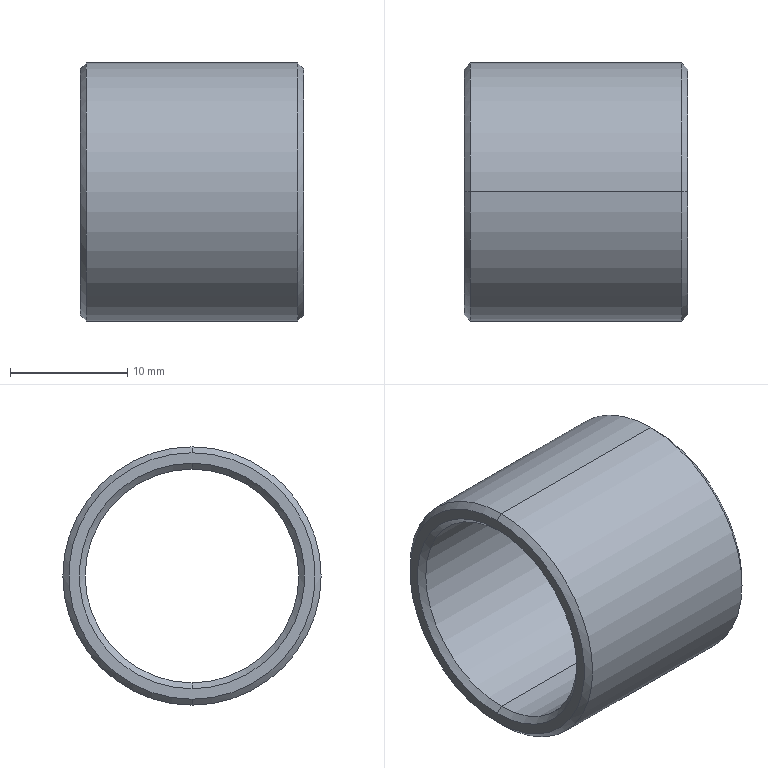Part | SolidWorks | features BaseBody 1 | 1 solid | 14 faces | box 19 x 22 x 22 mm | volume 2248 mm3 | cone 8 | cylinder 4 | plane 2 | commonest cylinder face diameters 18.2 x2 22 x2
STEP:
#1=CARTESIAN_POINT('',(100.647,1932.,-359.));
#2=VERTEX_POINT('',#1);
#3=CARTESIAN_POINT('',(100.647,1932.,-337.));
#4=VERTEX_POINT('',#3);
#5=CARTESIAN_POINT('',(100.647,1932.,-348.));
#6=DIRECTION('',(1.,0.,0.));
#7=DIRECTION('',(0.,0.,-1.));
#8=AXIS2_PLACEMENT_3D('',#5,#6,#7);
#9=CIRCLE('',#8,11.);
#10=EDGE_CURVE('',#2,#4,#9,.T.);
#11=ORIENTED_EDGE('',*,*,#10,.T.);
#12=CARTESIAN_POINT('',(118.647,1932.,-337.));
#13=VERTEX_POINT('',#12);
#14=CARTESIAN_POINT('',(100.147,1932.,-337.));
#15=DIRECTION('',(1.,0.,0.));
#16=VECTOR('',#15,1000.);
#17=LINE('',#14,#16);
#18=EDGE_CURVE('',#4,#13,#17,.T.);
#19=ORIENTED_EDGE('',*,*,#18,.T.);
#20=CARTESIAN_POINT('',(118.647,1932.,-359.));
#21=VERTEX_POINT('',#20);
#22=CARTESIAN_POINT('',(118.647,1932.,-348.));
#23=DIRECTION('',(-1.,0.,0.));
#24=DIRECTION('',(0.,0.,-1.));
#25=AXIS2_PLACEMENT_3D('',#22,#23,#24);
#26=CIRCLE('',#25,11.);
#27=EDGE_CURVE('',#13,#21,#26,.T.);
#28=ORIENTED_EDGE('',*,*,#27,.T.);
#29=CARTESIAN_POINT('',(100.147,1932.,-359.));
#30=DIRECTION('',(1.,0.,0.));
#31=VECTOR('',#30,1000.);
#32=LINE('',#29,#31);
#33=EDGE_CURVE('',#2,#21,#32,.T.);
#34=ORIENTED_EDGE('',*,*,#33,.F.);
#35=EDGE_LOOP('',(#11,#19,#28,#34));
#36=FACE_OUTER_BOUND('',#35,.T.);
#37=CARTESIAN_POINT('',(100.147,1932.,-348.));
#38=DIRECTION('',(1.,0.,0.));
#39=DIRECTION('',(0.,0.,-1.));
#40=AXIS2_PLACEMENT_3D('',#37,#38,#39);
#41=CYLINDRICAL_SURFACE('',#40,11.);
#42=ADVANCED_FACE('',(#36),#41,.T.);
#43=CARTESIAN_POINT('',(119.147,1932.,-337.5));
#44=VERTEX_POINT('',#43);
#45=CARTESIAN_POINT('',(119.147,1932.,-358.5));
#46=VERTEX_POINT('',#45);
#47=CARTESIAN_POINT('',(119.147,1932.,-348.));
#48=DIRECTION('',(-1.,0.,0.));
#49=DIRECTION('',(0.,0.,1.));
#50=AXIS2_PLACEMENT_3D('',#47,#48,#49);
#51=CIRCLE('',#50,10.5);
#52=EDGE_CURVE('',#44,#46,#51,.T.);
#53=ORIENTED_EDGE('',*,*,#52,.T.);
#54=CARTESIAN_POINT('',(118.647,1932.,-359.));
#55=DIRECTION('',(-0.7071,0.,-0.7071));
#56=VECTOR('',#55,1000.);
#57=LINE('',#54,#56);
#58=EDGE_CURVE('',#46,#21,#57,.T.);
#59=ORIENTED_EDGE('',*,*,#58,.T.);
#60=ORIENTED_EDGE('',*,*,#27,.F.);
#61=CARTESIAN_POINT('',(118.647,1932.,-337.));
#62=DIRECTION('',(-0.7071,0.,0.7071));
#63=VECTOR('',#62,1000.);
#64=LINE('',#61,#63);
#65=EDGE_CURVE('',#44,#13,#64,.T.);
#66=ORIENTED_EDGE('',*,*,#65,.F.);
#67=EDGE_LOOP('',(#53,#59,#60,#66));
#68=FACE_OUTER_BOUND('',#67,.T.);
#69=CARTESIAN_POINT('',(118.647,1932.,-348.));
#70=DIRECTION('',(-1.,0.,0.));
#71=DIRECTION('',(0.,0.,1.));
#72=AXIS2_PLACEMENT_3D('',#69,#70,#71);
#73=CONICAL_SURFACE('',#72,11.,0.7854);
#74=ADVANCED_FACE('',(#68),#73,.T.);
#75=CARTESIAN_POINT('',(100.147,1932.,-358.5));
#76=VERTEX_POINT('',#75);
#77=CARTESIAN_POINT('',(100.147,1932.,-337.5));
#78=VERTEX_POINT('',#77);
#79=CARTESIAN_POINT('',(100.147,1932.,-348.));
#80=DIRECTION('',(1.,0.,0.));
#81=DIRECTION('',(0.,0.,-1.));
#82=AXIS2_PLACEMENT_3D('',#79,#80,#81);
#83=CIRCLE('',#82,10.5);
#84=EDGE_CURVE('',#76,#78,#83,.T.);
#85=ORIENTED_EDGE('',*,*,#84,.T.);
#86=CARTESIAN_POINT('',(100.647,1932.,-337.));
#87=DIRECTION('',(0.7071,0.,0.7071));
#88=VECTOR('',#87,1000.);
#89=LINE('',#86,#88);
#90=EDGE_CURVE('',#78,#4,#89,.T.);
#91=ORIENTED_EDGE('',*,*,#90,.T.);
#92=ORIENTED_EDGE('',*,*,#10,.F.);
#93=CARTESIAN_POINT('',(100.647,1932.,-359.));
#94=DIRECTION('',(0.7071,0.,-0.7071));
#95=VECTOR('',#94,1000.);
#96=LINE('',#93,#95);
#97=EDGE_CURVE('',#76,#2,#96,.T.);
#98=ORIENTED_EDGE('',*,*,#97,.F.);
#99=EDGE_LOOP('',(#85,#91,#92,#98));
#100=FACE_OUTER_BOUND('',#99,.T.);
#101=CARTESIAN_POINT('',(100.647,1932.,-348.));
#102=DIRECTION('',(1.,0.,0.));
#103=DIRECTION('',(0.,0.,-1.));
#104=AXIS2_PLACEMENT_3D('',#101,#102,#103);
#105=CONICAL_SURFACE('',#104,11.,0.7854);
#106=ADVANCED_FACE('',(#100),#105,.T.);
#107=CARTESIAN_POINT('',(118.647,1932.,-338.9));
#108=VERTEX_POINT('',#107);
#109=CARTESIAN_POINT('',(118.647,1932.,-357.1));
#110=VERTEX_POINT('',#109);
#111=CARTESIAN_POINT('',(118.647,1932.,-348.));
#112=DIRECTION('',(1.,0.,0.));
#113=DIRECTION('',(0.,1.,0.));
#114=AXIS2_PLACEMENT_3D('',#111,#112,#113);
#115=CIRCLE('',#114,9.1);
#116=EDGE_CURVE('',#108,#110,#115,.T.);
#117=ORIENTED_EDGE('',*,*,#116,.F.);
#118=CARTESIAN_POINT('',(119.147,1932.,-338.4));
#119=VERTEX_POINT('',#118);
#120=CARTESIAN_POINT('',(119.147,1932.,-338.4));
#121=DIRECTION('',(0.7071,0.,0.7071));
#122=VECTOR('',#121,1000.);
#123=LINE('',#120,#122);
#124=EDGE_CURVE('',#108,#119,#123,.T.);
#125=ORIENTED_EDGE('',*,*,#124,.T.);
#126=CARTESIAN_POINT('',(119.147,1932.,-357.6));
#127=VERTEX_POINT('',#126);
#128=CARTESIAN_POINT('',(119.147,1932.,-348.));
#129=DIRECTION('',(1.,0.,0.));
#130=DIRECTION('',(0.,0.,-1.));
#131=AXIS2_PLACEMENT_3D('',#128,#129,#130);
#132=CIRCLE('',#131,9.6);
#133=EDGE_CURVE('',#119,#127,#132,.T.);
#134=ORIENTED_EDGE('',*,*,#133,.T.);
#135=CARTESIAN_POINT('',(119.147,1932.,-357.6));
#136=DIRECTION('',(0.7071,0.,-0.7071));
#137=VECTOR('',#136,1000.);
#138=LINE('',#135,#137);
#139=EDGE_CURVE('',#110,#127,#138,.T.);
#140=ORIENTED_EDGE('',*,*,#139,.F.);
#141=EDGE_LOOP('',(#117,#125,#134,#140));
#142=FACE_OUTER_BOUND('',#141,.T.);
#143=CARTESIAN_POINT('',(119.147,1932.,-348.));
#144=DIRECTION('',(1.,0.,0.));
#145=DIRECTION('',(0.,0.,-1.));
#146=AXIS2_PLACEMENT_3D('',#143,#144,#145);
#147=CONICAL_SURFACE('',#146,9.6,0.7854);
#148=ADVANCED_FACE('',(#142),#147,.F.);
#149=CARTESIAN_POINT('',(100.647,1932.,-357.1));
#150=VERTEX_POINT('',#149);
#151=CARTESIAN_POINT('',(100.647,1932.,-338.9));
#152=VERTEX_POINT('',#151);
#153=CARTESIAN_POINT('',(100.647,1932.,-348.));
#154=DIRECTION('',(-1.,0.,0.));
#155=DIRECTION('',(0.,-1.,0.));
#156=AXIS2_PLACEMENT_3D('',#153,#154,#155);
#157=CIRCLE('',#156,9.1);
#158=EDGE_CURVE('',#150,#152,#157,.T.);
#159=ORIENTED_EDGE('',*,*,#158,.F.);
#160=CARTESIAN_POINT('',(100.147,1932.,-357.6));
#161=VERTEX_POINT('',#160);
#162=CARTESIAN_POINT('',(100.147,1932.,-357.6));
#163=DIRECTION('',(-0.7071,0.,-0.7071));
#164=VECTOR('',#163,1000.);
#165=LINE('',#162,#164);
#166=EDGE_CURVE('',#150,#161,#165,.T.);
#167=ORIENTED_EDGE('',*,*,#166,.T.);
#168=CARTESIAN_POINT('',(100.147,1932.,-338.4));
#169=VERTEX_POINT('',#168);
#170=CARTESIAN_POINT('',(100.147,1932.,-348.));
#171=DIRECTION('',(1.,0.,0.));
#172=DIRECTION('',(0.,0.,1.));
#173=AXIS2_PLACEMENT_3D('',#170,#171,#172);
#174=CIRCLE('',#173,9.6);
#175=EDGE_CURVE('',#169,#161,#174,.T.);
#176=ORIENTED_EDGE('',*,*,#175,.F.);
#177=CARTESIAN_POINT('',(100.147,1932.,-338.4));
#178=DIRECTION('',(-0.7071,0.,0.7071));
#179=VECTOR('',#178,1000.);
#180=LINE('',#177,#179);
#181=EDGE_CURVE('',#152,#169,#180,.T.);
#182=ORIENTED_EDGE('',*,*,#181,.F.);
#183=EDGE_LOOP('',(#159,#167,#176,#182));
#184=FACE_OUTER_BOUND('',#183,.T.);
#185=CARTESIAN_POINT('',(100.147,1932.,-348.));
#186=DIRECTION('',(-1.,0.,0.));
#187=DIRECTION('',(0.,0.,1.));
#188=AXIS2_PLACEMENT_3D('',#185,#186,#187);
#189=CONICAL_SURFACE('',#188,9.6,0.7854);
#190=ADVANCED_FACE('',(#184),#189,.F.);
#191=ORIENTED_EDGE('',*,*,#158,.T.);
#192=CARTESIAN_POINT('',(100.147,1932.,-338.9));
#193=DIRECTION('',(1.,0.,0.));
#194=VECTOR('',#193,1000.);
#195=LINE('',#192,#194);
#196=EDGE_CURVE('',#152,#108,#195,.T.);
#197=ORIENTED_EDGE('',*,*,#196,.T.);
#198=ORIENTED_EDGE('',*,*,#116,.T.);
#199=CARTESIAN_POINT('',(100.147,1932.,-357.1));
#200=DIRECTION('',(1.,0.,0.));
#201=VECTOR('',#200,1000.);
#202=LINE('',#199,#201);
#203=EDGE_CURVE('',#150,#110,#202,.T.);
#204=ORIENTED_EDGE('',*,*,#203,.F.);
#205=EDGE_LOOP('',(#191,#197,#198,#204));
#206=FACE_OUTER_BOUND('',#205,.T.);
#207=CARTESIAN_POINT('',(100.147,1932.,-348.));
#208=DIRECTION('',(1.,0.,0.));
#209=DIRECTION('',(0.,0.,-1.));
#210=AXIS2_PLACEMENT_3D('',#207,#208,#209);
#211=CYLINDRICAL_SURFACE('',#210,9.1);
#212=ADVANCED_FACE('',(#206),#211,.F.);
#213=ORIENTED_EDGE('',*,*,#18,.F.);
#214=CARTESIAN_POINT('',(100.647,1932.,-348.));
#215=DIRECTION('',(1.,0.,0.));
#216=DIRECTION('',(0.,0.,-1.));
#217=AXIS2_PLACEMENT_3D('',#214,#215,#216);
#218=CIRCLE('',#217,11.);
#219=EDGE_CURVE('',#4,#2,#218,.T.);
#220=ORIENTED_EDGE('',*,*,#219,.T.);
#221=ORIENTED_EDGE('',*,*,#33,.T.);
#222=CARTESIAN_POINT('',(118.647,1932.,-348.));
#223=DIRECTION('',(-1.,0.,0.));
#224=DIRECTION('',(0.,0.,-1.));
#225=AXIS2_PLACEMENT_3D('',#222,#223,#224);
#226=CIRCLE('',#225,11.);
#227=EDGE_CURVE('',#21,#13,#226,.T.);
#228=ORIENTED_EDGE('',*,*,#227,.T.);
#229=EDGE_LOOP('',(#213,#220,#221,#228));
#230=FACE_OUTER_BOUND('',#229,.T.);
#231=CARTESIAN_POINT('',(100.147,1932.,-348.));
#232=DIRECTION('',(1.,0.,0.));
#233=DIRECTION('',(0.,0.,-1.));
#234=AXIS2_PLACEMENT_3D('',#231,#232,#233);
#235=CYLINDRICAL_SURFACE('',#234,11.);
#236=ADVANCED_FACE('',(#230),#235,.T.);
#237=ORIENTED_EDGE('',*,*,#58,.F.);
#238=CARTESIAN_POINT('',(119.147,1932.,-348.));
#239=DIRECTION('',(-1.,0.,0.));
#240=DIRECTION('',(0.,0.,1.));
#241=AXIS2_PLACEMENT_3D('',#238,#239,#240);
#242=CIRCLE('',#241,10.5);
#243=EDGE_CURVE('',#46,#44,#242,.T.);
#244=ORIENTED_EDGE('',*,*,#243,.T.);
#245=ORIENTED_EDGE('',*,*,#65,.T.);
#246=ORIENTED_EDGE('',*,*,#227,.F.);
#247=EDGE_LOOP('',(#237,#244,#245,#246));
#248=FACE_OUTER_BOUND('',#247,.T.);
#249=CARTESIAN_POINT('',(118.647,1932.,-348.));
#250=DIRECTION('',(-1.,0.,0.));
#251=DIRECTION('',(0.,0.,1.));
#252=AXIS2_PLACEMENT_3D('',#249,#250,#251);
#253=CONICAL_SURFACE('',#252,11.,0.7854);
#254=ADVANCED_FACE('',(#248),#253,.T.);
#255=ORIENTED_EDGE('',*,*,#90,.F.);
#256=CARTESIAN_POINT('',(100.147,1932.,-348.));
#257=DIRECTION('',(1.,0.,0.));
#258=DIRECTION('',(0.,0.,-1.));
#259=AXIS2_PLACEMENT_3D('',#256,#257,#258);
#260=CIRCLE('',#259,10.5);
#261=EDGE_CURVE('',#78,#76,#260,.T.);
#262=ORIENTED_EDGE('',*,*,#261,.T.);
#263=ORIENTED_EDGE('',*,*,#97,.T.);
#264=ORIENTED_EDGE('',*,*,#219,.F.);
#265=EDGE_LOOP('',(#255,#262,#263,#264));
#266=FACE_OUTER_BOUND('',#265,.T.);
#267=CARTESIAN_POINT('',(100.647,1932.,-348.));
#268=DIRECTION('',(1.,0.,0.));
#269=DIRECTION('',(0.,0.,-1.));
#270=AXIS2_PLACEMENT_3D('',#267,#268,#269);
#271=CONICAL_SURFACE('',#270,11.,0.7854);
#272=ADVANCED_FACE('',(#266),#271,.T.);
#273=CARTESIAN_POINT('',(119.147,1932.,-348.));
#274=DIRECTION('',(1.,0.,0.));
#275=DIRECTION('',(0.,0.,-1.));
#276=AXIS2_PLACEMENT_3D('',#273,#274,#275);
#277=CIRCLE('',#276,9.6);
#278=EDGE_CURVE('',#127,#119,#277,.T.);
#279=ORIENTED_EDGE('',*,*,#278,.F.);
#280=ORIENTED_EDGE('',*,*,#133,.F.);
#281=EDGE_LOOP('',(#279,#280));
#282=FACE_BOUND('',#281,.T.);
#283=ORIENTED_EDGE('',*,*,#52,.F.);
#284=ORIENTED_EDGE('',*,*,#243,.F.);
#285=EDGE_LOOP('',(#283,#284));
#286=FACE_OUTER_BOUND('',#285,.T.);
#287=CARTESIAN_POINT('',(119.147,1932.,-348.));
#288=DIRECTION('',(-1.,0.,0.));
#289=DIRECTION('',(0.,0.,1.));
#290=AXIS2_PLACEMENT_3D('',#287,#288,#289);
#291=PLANE('',#290);
#292=ADVANCED_FACE('',(#282,#286),#291,.F.);
#293=ORIENTED_EDGE('',*,*,#175,.T.);
#294=CARTESIAN_POINT('',(100.147,1932.,-348.));
#295=DIRECTION('',(1.,0.,0.));
#296=DIRECTION('',(0.,0.,1.));
#297=AXIS2_PLACEMENT_3D('',#294,#295,#296);
#298=CIRCLE('',#297,9.6);
#299=EDGE_CURVE('',#161,#169,#298,.T.);
#300=ORIENTED_EDGE('',*,*,#299,.T.);
#301=EDGE_LOOP('',(#293,#300));
#302=FACE_BOUND('',#301,.T.);
#303=ORIENTED_EDGE('',*,*,#84,.F.);
#304=ORIENTED_EDGE('',*,*,#261,.F.);
#305=EDGE_LOOP('',(#303,#304));
#306=FACE_OUTER_BOUND('',#305,.T.);
#307=CARTESIAN_POINT('',(100.147,1932.,-348.));
#308=DIRECTION('',(-1.,0.,0.));
#309=DIRECTION('',(0.,0.,1.));
#310=AXIS2_PLACEMENT_3D('',#307,#308,#309);
#311=PLANE('',#310);
#312=ADVANCED_FACE('',(#302,#306),#311,.T.);
#313=ORIENTED_EDGE('',*,*,#124,.F.);
#314=CARTESIAN_POINT('',(118.647,1932.,-348.));
#315=DIRECTION('',(1.,0.,0.));
#316=DIRECTION('',(0.,1.,0.));
#317=AXIS2_PLACEMENT_3D('',#314,#315,#316);
#318=CIRCLE('',#317,9.1);
#319=EDGE_CURVE('',#110,#108,#318,.T.);
#320=ORIENTED_EDGE('',*,*,#319,.F.);
#321=ORIENTED_EDGE('',*,*,#139,.T.);
#322=ORIENTED_EDGE('',*,*,#278,.T.);
#323=EDGE_LOOP('',(#313,#320,#321,#322));
#324=FACE_OUTER_BOUND('',#323,.T.);
#325=CARTESIAN_POINT('',(119.147,1932.,-348.));
#326=DIRECTION('',(1.,0.,0.));
#327=DIRECTION('',(0.,0.,-1.));
#328=AXIS2_PLACEMENT_3D('',#325,#326,#327);
#329=CONICAL_SURFACE('',#328,9.6,0.7854);
#330=ADVANCED_FACE('',(#324),#329,.F.);
#331=ORIENTED_EDGE('',*,*,#166,.F.);
#332=CARTESIAN_POINT('',(100.647,1932.,-348.));
#333=DIRECTION('',(-1.,0.,0.));
#334=DIRECTION('',(0.,-1.,0.));
#335=AXIS2_PLACEMENT_3D('',#332,#333,#334);
#336=CIRCLE('',#335,9.1);
#337=EDGE_CURVE('',#152,#150,#336,.T.);
#338=ORIENTED_EDGE('',*,*,#337,.F.);
#339=ORIENTED_EDGE('',*,*,#181,.T.);
#340=ORIENTED_EDGE('',*,*,#299,.F.);
#341=EDGE_LOOP('',(#331,#338,#339,#340));
#342=FACE_OUTER_BOUND('',#341,.T.);
#343=CARTESIAN_POINT('',(100.147,1932.,-348.));
#344=DIRECTION('',(-1.,0.,0.));
#345=DIRECTION('',(0.,0.,1.));
#346=AXIS2_PLACEMENT_3D('',#343,#344,#345);
#347=CONICAL_SURFACE('',#346,9.6,0.7854);
#348=ADVANCED_FACE('',(#342),#347,.F.);
#349=ORIENTED_EDGE('',*,*,#196,.F.);
#350=ORIENTED_EDGE('',*,*,#337,.T.);
#351=ORIENTED_EDGE('',*,*,#203,.T.);
#352=ORIENTED_EDGE('',*,*,#319,.T.);
#353=EDGE_LOOP('',(#349,#350,#351,#352));
#354=FACE_OUTER_BOUND('',#353,.T.);
#355=CARTESIAN_POINT('',(100.147,1932.,-348.));
#356=DIRECTION('',(1.,0.,0.));
#357=DIRECTION('',(0.,0.,-1.));
#358=AXIS2_PLACEMENT_3D('',#355,#356,#357);
#359=CYLINDRICAL_SURFACE('',#358,9.1);
#360=ADVANCED_FACE('',(#354),#359,.F.);
#361=CLOSED_SHELL('',(#42,#74,#106,#148,#190,#212,#236,#254,#272,#292,#312,#330,#348,#360));
#362=MANIFOLD_SOLID_BREP('',#361);
#363=CARTESIAN_POINT('',(0.,0.,0.));
#364=DIRECTION('',(0.,0.,1.));
#365=DIRECTION('',(1.,0.,0.));
#366=AXIS2_PLACEMENT_3D('',#363,#364,#365);
#367=(LENGTH_UNIT()NAMED_UNIT(*)SI_UNIT(.MILLI.,.METRE.));
#368=UNCERTAINTY_MEASURE_WITH_UNIT(LENGTH_MEASURE(0.00001),#367,'','');
#369=(NAMED_UNIT(*)PLANE_ANGLE_UNIT()SI_UNIT($,.RADIAN.));
#370=(NAMED_UNIT(*)SI_UNIT($,.STERADIAN.)SOLID_ANGLE_UNIT());
#371=(GEOMETRIC_REPRESENTATION_CONTEXT(3)GLOBAL_UNCERTAINTY_ASSIGNED_CONTEXT((#368))GLOBAL_UNIT_ASSIGNED_CONTEXT((#367,#369,#370))REPRESENTATION_CONTEXT('',''));
#372=ADVANCED_BREP_SHAPE_REPRESENTATION('',(#362,#366),#371);